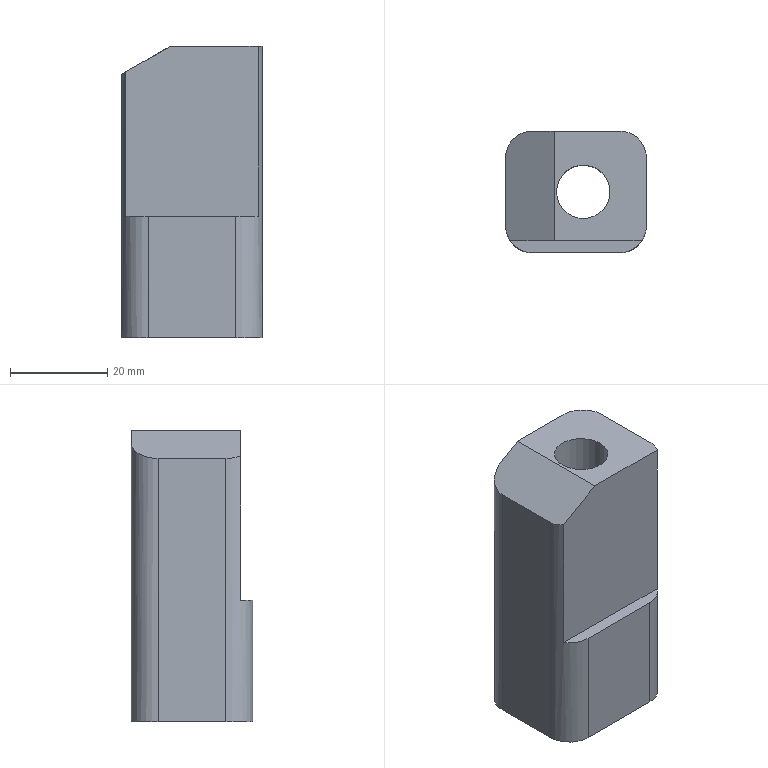Part | NX | features 1605338300 2 | 1 solid | 16 faces | box 29 x 25 x 60 mm | volume 29922 mm3 | plane 10 | cylinder 6 | commonest cylinder face diameters 11 x5 17 x1
STEP:
#1=CARTESIAN_POINT('',(321.5,0.000000002,-34.5));
#2=VERTEX_POINT('',#1);
#3=CARTESIAN_POINT('',(330.,0.000000002,-34.5));
#4=DIRECTION('',(0.,0.,-1.));
#5=DIRECTION('',(-1.,0.,0.));
#6=AXIS2_PLACEMENT_3D('',#3,#4,#5);
#7=CIRCLE('',#6,8.5);
#8=EDGE_CURVE('',#2,#2,#7,.T.);
#9=ORIENTED_EDGE('',*,*,#8,.F.);
#10=EDGE_LOOP('',(#9));
#11=FACE_BOUND('',#10,.T.);
#12=CARTESIAN_POINT('',(321.5,0.000000002,-61.5));
#13=VERTEX_POINT('',#12);
#14=CARTESIAN_POINT('',(330.,0.000000002,-61.5));
#15=DIRECTION('',(0.,0.,-1.));
#16=DIRECTION('',(-1.,0.,0.));
#17=AXIS2_PLACEMENT_3D('',#14,#15,#16);
#18=CIRCLE('',#17,8.5);
#19=EDGE_CURVE('',#13,#13,#18,.F.);
#20=ORIENTED_EDGE('',*,*,#19,.F.);
#21=EDGE_LOOP('',(#20));
#22=FACE_BOUND('',#21,.T.);
#23=CARTESIAN_POINT('',(330.,0.000000002,-34.5));
#24=DIRECTION('',(0.,0.,-1.));
#25=DIRECTION('',(-1.,0.,0.));
#26=AXIS2_PLACEMENT_3D('',#23,#24,#25);
#27=CYLINDRICAL_SURFACE('',#26,8.5);
#28=ADVANCED_FACE('',(#11,#22),#27,.F.);
#29=CARTESIAN_POINT('',(324.5,0.,-34.5));
#30=VERTEX_POINT('',#29);
#31=CARTESIAN_POINT('',(330.,0.,-34.5));
#32=DIRECTION('',(0.,0.,-1.));
#33=DIRECTION('',(-1.,0.,0.));
#34=AXIS2_PLACEMENT_3D('',#31,#32,#33);
#35=CIRCLE('',#34,5.5);
#36=EDGE_CURVE('',#30,#30,#35,.T.);
#37=ORIENTED_EDGE('',*,*,#36,.T.);
#38=EDGE_LOOP('',(#37));
#39=FACE_BOUND('',#38,.T.);
#40=CARTESIAN_POINT('',(335.5,0.,-1.5));
#41=VERTEX_POINT('',#40);
#42=CARTESIAN_POINT('',(330.,0.,-1.5));
#43=DIRECTION('',(0.,0.,1.));
#44=DIRECTION('',(1.,0.,0.));
#45=AXIS2_PLACEMENT_3D('',#42,#43,#44);
#46=CIRCLE('',#45,5.5);
#47=EDGE_CURVE('',#41,#41,#46,.F.);
#48=ORIENTED_EDGE('',*,*,#47,.F.);
#49=EDGE_LOOP('',(#48));
#50=FACE_BOUND('',#49,.T.);
#51=CARTESIAN_POINT('',(330.,0.,20.5));
#52=DIRECTION('',(0.,0.,-1.));
#53=DIRECTION('',(-1.,0.,0.));
#54=AXIS2_PLACEMENT_3D('',#51,#52,#53);
#55=CYLINDRICAL_SURFACE('',#54,5.5);
#56=ADVANCED_FACE('',(#39,#50),#55,.F.);
#57=CARTESIAN_POINT('',(324.,-10.,-1.5));
#58=VERTEX_POINT('',#57);
#59=CARTESIAN_POINT('',(324.,12.5,-1.5));
#60=VERTEX_POINT('',#59);
#61=CARTESIAN_POINT('',(324.,-5.,-1.5));
#62=DIRECTION('',(0.,1.,0.));
#63=VECTOR('',#62,1000.);
#64=LINE('',#61,#63);
#65=EDGE_CURVE('',#58,#60,#64,.T.);
#66=ORIENTED_EDGE('',*,*,#65,.F.);
#67=CARTESIAN_POINT('',(342.11,-10.,-1.5));
#68=VERTEX_POINT('',#67);
#69=CARTESIAN_POINT('',(326.,-10.,-1.5));
#70=DIRECTION('',(1.,0.,0.));
#71=VECTOR('',#70,1000.);
#72=LINE('',#69,#71);
#73=EDGE_CURVE('',#58,#68,#72,.T.);
#74=ORIENTED_EDGE('',*,*,#73,.T.);
#75=CARTESIAN_POINT('',(343.,-7.,-1.5));
#76=VERTEX_POINT('',#75);
#77=CARTESIAN_POINT('',(337.5,-7.,-1.5));
#78=DIRECTION('',(0.,0.,1.));
#79=DIRECTION('',(1.,0.,0.));
#80=AXIS2_PLACEMENT_3D('',#77,#78,#79);
#81=CIRCLE('',#80,5.5);
#82=EDGE_CURVE('',#76,#68,#81,.F.);
#83=ORIENTED_EDGE('',*,*,#82,.F.);
#84=CARTESIAN_POINT('',(343.,7.,-1.5));
#85=VERTEX_POINT('',#84);
#86=CARTESIAN_POINT('',(343.,-5.,-1.5));
#87=DIRECTION('',(0.,1.,0.));
#88=VECTOR('',#87,1000.);
#89=LINE('',#86,#88);
#90=EDGE_CURVE('',#76,#85,#89,.T.);
#91=ORIENTED_EDGE('',*,*,#90,.T.);
#92=CARTESIAN_POINT('',(337.5,12.5,-1.5));
#93=VERTEX_POINT('',#92);
#94=CARTESIAN_POINT('',(337.5,7.,-1.5));
#95=DIRECTION('',(0.,0.,1.));
#96=DIRECTION('',(1.,0.,0.));
#97=AXIS2_PLACEMENT_3D('',#94,#95,#96);
#98=CIRCLE('',#97,5.5);
#99=EDGE_CURVE('',#93,#85,#98,.F.);
#100=ORIENTED_EDGE('',*,*,#99,.F.);
#101=CARTESIAN_POINT('',(299.,12.5,-1.5));
#102=DIRECTION('',(-1.,0.,0.));
#103=VECTOR('',#102,1000.);
#104=LINE('',#101,#103);
#105=EDGE_CURVE('',#93,#60,#104,.T.);
#106=ORIENTED_EDGE('',*,*,#105,.T.);
#107=EDGE_LOOP('',(#66,#74,#83,#91,#100,#106));
#108=FACE_BOUND('',#107,.T.);
#109=ORIENTED_EDGE('',*,*,#47,.T.);
#110=EDGE_LOOP('',(#109));
#111=FACE_BOUND('',#110,.T.);
#112=CARTESIAN_POINT('',(299.,-5.,-1.5));
#113=DIRECTION('',(0.,0.,1.));
#114=DIRECTION('',(1.,0.,0.));
#115=AXIS2_PLACEMENT_3D('',#112,#113,#114);
#116=PLANE('',#115);
#117=ADVANCED_FACE('',(#108,#111),#116,.T.);
#118=CARTESIAN_POINT('',(337.5,-12.5,-36.5));
#119=VERTEX_POINT('',#118);
#120=CARTESIAN_POINT('',(319.5,-12.5,-36.5));
#121=VERTEX_POINT('',#120);
#122=CARTESIAN_POINT('',(326.,-12.5,-36.5));
#123=DIRECTION('',(1.,0.,0.));
#124=VECTOR('',#123,1000.);
#125=LINE('',#122,#124);
#126=EDGE_CURVE('',#119,#121,#125,.F.);
#127=ORIENTED_EDGE('',*,*,#126,.T.);
#128=CARTESIAN_POINT('',(319.5,-12.5,-61.5));
#129=VERTEX_POINT('',#128);
#130=CARTESIAN_POINT('',(319.5,-12.5,-1.5));
#131=DIRECTION('',(0.,0.,-1.));
#132=VECTOR('',#131,1000.);
#133=LINE('',#130,#132);
#134=EDGE_CURVE('',#129,#121,#133,.F.);
#135=ORIENTED_EDGE('',*,*,#134,.F.);
#136=CARTESIAN_POINT('',(337.5,-12.5,-61.5));
#137=VERTEX_POINT('',#136);
#138=CARTESIAN_POINT('',(299.,-12.5,-61.5));
#139=DIRECTION('',(-1.,0.,0.));
#140=VECTOR('',#139,1000.);
#141=LINE('',#138,#140);
#142=EDGE_CURVE('',#137,#129,#141,.T.);
#143=ORIENTED_EDGE('',*,*,#142,.F.);
#144=CARTESIAN_POINT('',(337.5,-12.5,-1.5));
#145=DIRECTION('',(0.,0.,-1.));
#146=VECTOR('',#145,1000.);
#147=LINE('',#144,#146);
#148=EDGE_CURVE('',#119,#137,#147,.T.);
#149=ORIENTED_EDGE('',*,*,#148,.F.);
#150=EDGE_LOOP('',(#127,#135,#143,#149));
#151=FACE_BOUND('',#150,.T.);
#152=CARTESIAN_POINT('',(299.,-12.5,-1.5));
#153=DIRECTION('',(0.,-1.,0.));
#154=DIRECTION('',(0.,0.,1.));
#155=AXIS2_PLACEMENT_3D('',#152,#153,#154);
#156=PLANE('',#155);
#157=ADVANCED_FACE('',(#151),#156,.T.);
#158=CARTESIAN_POINT('',(314.,7.,-7.274));
#159=VERTEX_POINT('',#158);
#160=CARTESIAN_POINT('',(314.,-7.,-7.274));
#161=VERTEX_POINT('',#160);
#162=CARTESIAN_POINT('',(314.,-5.,-7.274));
#163=DIRECTION('',(0.,1.,0.));
#164=VECTOR('',#163,1000.);
#165=LINE('',#162,#164);
#166=EDGE_CURVE('',#159,#161,#165,.F.);
#167=ORIENTED_EDGE('',*,*,#166,.F.);
#168=CARTESIAN_POINT('',(314.,7.,-61.5));
#169=VERTEX_POINT('',#168);
#170=CARTESIAN_POINT('',(314.,7.,-1.5));
#171=DIRECTION('',(0.,0.,-1.));
#172=VECTOR('',#171,1000.);
#173=LINE('',#170,#172);
#174=EDGE_CURVE('',#169,#159,#173,.F.);
#175=ORIENTED_EDGE('',*,*,#174,.F.);
#176=CARTESIAN_POINT('',(314.,-7.,-61.5));
#177=VERTEX_POINT('',#176);
#178=CARTESIAN_POINT('',(314.,-5.,-61.5));
#179=DIRECTION('',(0.,1.,0.));
#180=VECTOR('',#179,1000.);
#181=LINE('',#178,#180);
#182=EDGE_CURVE('',#177,#169,#181,.T.);
#183=ORIENTED_EDGE('',*,*,#182,.F.);
#184=CARTESIAN_POINT('',(314.,-7.,-1.5));
#185=DIRECTION('',(0.,0.,-1.));
#186=VECTOR('',#185,1000.);
#187=LINE('',#184,#186);
#188=EDGE_CURVE('',#161,#177,#187,.T.);
#189=ORIENTED_EDGE('',*,*,#188,.F.);
#190=EDGE_LOOP('',(#167,#175,#183,#189));
#191=FACE_BOUND('',#190,.T.);
#192=CARTESIAN_POINT('',(314.,-5.,-1.5));
#193=DIRECTION('',(-1.,0.,0.));
#194=DIRECTION('',(0.,0.,1.));
#195=AXIS2_PLACEMENT_3D('',#192,#193,#194);
#196=PLANE('',#195);
#197=ADVANCED_FACE('',(#191),#196,.T.);
#198=CARTESIAN_POINT('',(319.5,12.5,-4.098));
#199=VERTEX_POINT('',#198);
#200=CARTESIAN_POINT('',(301.5,12.5,-14.49));
#201=DIRECTION('',(-0.866,0.,-0.5));
#202=VECTOR('',#201,1000.);
#203=LINE('',#200,#202);
#204=EDGE_CURVE('',#60,#199,#203,.T.);
#205=ORIENTED_EDGE('',*,*,#204,.F.);
#206=ORIENTED_EDGE('',*,*,#105,.F.);
#207=CARTESIAN_POINT('',(337.5,12.5,-61.5));
#208=VERTEX_POINT('',#207);
#209=CARTESIAN_POINT('',(337.5,12.5,-1.5));
#210=DIRECTION('',(0.,0.,-1.));
#211=VECTOR('',#210,1000.);
#212=LINE('',#209,#211);
#213=EDGE_CURVE('',#208,#93,#212,.F.);
#214=ORIENTED_EDGE('',*,*,#213,.F.);
#215=CARTESIAN_POINT('',(319.5,12.5,-61.5));
#216=VERTEX_POINT('',#215);
#217=CARTESIAN_POINT('',(299.,12.5,-61.5));
#218=DIRECTION('',(1.,0.,0.));
#219=VECTOR('',#218,1000.);
#220=LINE('',#217,#219);
#221=EDGE_CURVE('',#216,#208,#220,.T.);
#222=ORIENTED_EDGE('',*,*,#221,.F.);
#223=CARTESIAN_POINT('',(319.5,12.5,-1.5));
#224=DIRECTION('',(0.,0.,-1.));
#225=VECTOR('',#224,1000.);
#226=LINE('',#223,#225);
#227=EDGE_CURVE('',#199,#216,#226,.T.);
#228=ORIENTED_EDGE('',*,*,#227,.F.);
#229=EDGE_LOOP('',(#205,#206,#214,#222,#228));
#230=FACE_BOUND('',#229,.T.);
#231=CARTESIAN_POINT('',(299.,12.5,-1.5));
#232=DIRECTION('',(0.,1.,0.));
#233=DIRECTION('',(0.,0.,-1.));
#234=AXIS2_PLACEMENT_3D('',#231,#232,#233);
#235=PLANE('',#234);
#236=ADVANCED_FACE('',(#230),#235,.T.);
#237=CARTESIAN_POINT('',(343.,7.,-61.5));
#238=VERTEX_POINT('',#237);
#239=CARTESIAN_POINT('',(343.,-7.,-61.5));
#240=VERTEX_POINT('',#239);
#241=CARTESIAN_POINT('',(343.,-5.,-61.5));
#242=DIRECTION('',(0.,-1.,0.));
#243=VECTOR('',#242,1000.);
#244=LINE('',#241,#243);
#245=EDGE_CURVE('',#238,#240,#244,.T.);
#246=ORIENTED_EDGE('',*,*,#245,.F.);
#247=CARTESIAN_POINT('',(343.,7.,-1.5));
#248=DIRECTION('',(0.,0.,-1.));
#249=VECTOR('',#248,1000.);
#250=LINE('',#247,#249);
#251=EDGE_CURVE('',#85,#238,#250,.T.);
#252=ORIENTED_EDGE('',*,*,#251,.F.);
#253=ORIENTED_EDGE('',*,*,#90,.F.);
#254=CARTESIAN_POINT('',(343.,-7.,-1.5));
#255=DIRECTION('',(0.,0.,-1.));
#256=VECTOR('',#255,1000.);
#257=LINE('',#254,#256);
#258=EDGE_CURVE('',#240,#76,#257,.F.);
#259=ORIENTED_EDGE('',*,*,#258,.F.);
#260=EDGE_LOOP('',(#246,#252,#253,#259));
#261=FACE_BOUND('',#260,.T.);
#262=CARTESIAN_POINT('',(343.,-5.,-1.5));
#263=DIRECTION('',(1.,0.,0.));
#264=DIRECTION('',(0.,0.,-1.));
#265=AXIS2_PLACEMENT_3D('',#262,#263,#264);
#266=PLANE('',#265);
#267=ADVANCED_FACE('',(#261),#266,.T.);
#268=CARTESIAN_POINT('',(314.89,-10.,-6.76));
#269=VERTEX_POINT('',#268);
#270=CARTESIAN_POINT('',(314.,-10.,-7.274));
#271=DIRECTION('',(0.866,0.,0.5));
#272=VECTOR('',#271,1000.);
#273=LINE('',#270,#272);
#274=EDGE_CURVE('',#58,#269,#273,.F.);
#275=ORIENTED_EDGE('',*,*,#274,.F.);
#276=ORIENTED_EDGE('',*,*,#65,.T.);
#277=ORIENTED_EDGE('',*,*,#204,.T.);
#278=CARTESIAN_POINT('',(319.5,7.,-4.098));
#279=DIRECTION('',(0.5,0.,-0.866));
#280=DIRECTION('',(0.866,0.,0.5));
#281=AXIS2_PLACEMENT_3D('',#278,#279,#280);
#282=ELLIPSE('',#281,6.351,5.5);
#283=EDGE_CURVE('',#159,#199,#282,.T.);
#284=ORIENTED_EDGE('',*,*,#283,.F.);
#285=ORIENTED_EDGE('',*,*,#166,.T.);
#286=CARTESIAN_POINT('',(319.5,-7.,-4.098));
#287=DIRECTION('',(0.5,0.,-0.866));
#288=DIRECTION('',(0.866,0.,0.5));
#289=AXIS2_PLACEMENT_3D('',#286,#287,#288);
#290=ELLIPSE('',#289,6.351,5.5);
#291=EDGE_CURVE('',#269,#161,#290,.T.);
#292=ORIENTED_EDGE('',*,*,#291,.F.);
#293=EDGE_LOOP('',(#275,#276,#277,#284,#285,#292));
#294=FACE_BOUND('',#293,.T.);
#295=CARTESIAN_POINT('',(314.,-5.,-7.274));
#296=DIRECTION('',(0.5,0.,-0.866));
#297=DIRECTION('',(-0.866,0.,-0.5));
#298=AXIS2_PLACEMENT_3D('',#295,#296,#297);
#299=PLANE('',#298);
#300=ADVANCED_FACE('',(#294),#299,.F.);
#301=ORIENTED_EDGE('',*,*,#99,.T.);
#302=ORIENTED_EDGE('',*,*,#251,.T.);
#303=CARTESIAN_POINT('',(337.5,7.,-61.5));
#304=DIRECTION('',(0.,0.,-1.));
#305=DIRECTION('',(-1.,0.,0.));
#306=AXIS2_PLACEMENT_3D('',#303,#304,#305);
#307=CIRCLE('',#306,5.5);
#308=EDGE_CURVE('',#238,#208,#307,.F.);
#309=ORIENTED_EDGE('',*,*,#308,.T.);
#310=ORIENTED_EDGE('',*,*,#213,.T.);
#311=EDGE_LOOP('',(#301,#302,#309,#310));
#312=FACE_BOUND('',#311,.T.);
#313=CARTESIAN_POINT('',(337.5,7.,-1.5));
#314=DIRECTION('',(0.,0.,1.));
#315=DIRECTION('',(1.,0.,0.));
#316=AXIS2_PLACEMENT_3D('',#313,#314,#315);
#317=CYLINDRICAL_SURFACE('',#316,5.5);
#318=ADVANCED_FACE('',(#312),#317,.T.);
#319=CARTESIAN_POINT('',(342.11,-10.,-36.5));
#320=VERTEX_POINT('',#319);
#321=CARTESIAN_POINT('',(337.5,-7.,-36.5));
#322=DIRECTION('',(0.,0.,1.));
#323=DIRECTION('',(1.,0.,0.));
#324=AXIS2_PLACEMENT_3D('',#321,#322,#323);
#325=CIRCLE('',#324,5.5);
#326=EDGE_CURVE('',#320,#119,#325,.F.);
#327=ORIENTED_EDGE('',*,*,#326,.T.);
#328=ORIENTED_EDGE('',*,*,#148,.T.);
#329=CARTESIAN_POINT('',(337.5,-7.,-61.5));
#330=DIRECTION('',(0.,0.,-1.));
#331=DIRECTION('',(-1.,0.,0.));
#332=AXIS2_PLACEMENT_3D('',#329,#330,#331);
#333=CIRCLE('',#332,5.5);
#334=EDGE_CURVE('',#137,#240,#333,.F.);
#335=ORIENTED_EDGE('',*,*,#334,.T.);
#336=ORIENTED_EDGE('',*,*,#258,.T.);
#337=ORIENTED_EDGE('',*,*,#82,.T.);
#338=CARTESIAN_POINT('',(342.11,-10.,-1.5));
#339=DIRECTION('',(0.,0.,1.));
#340=VECTOR('',#339,1000.);
#341=LINE('',#338,#340);
#342=EDGE_CURVE('',#68,#320,#341,.F.);
#343=ORIENTED_EDGE('',*,*,#342,.T.);
#344=EDGE_LOOP('',(#327,#328,#335,#336,#337,#343));
#345=FACE_BOUND('',#344,.T.);
#346=CARTESIAN_POINT('',(337.5,-7.,-1.5));
#347=DIRECTION('',(0.,0.,1.));
#348=DIRECTION('',(1.,0.,0.));
#349=AXIS2_PLACEMENT_3D('',#346,#347,#348);
#350=CYLINDRICAL_SURFACE('',#349,5.5);
#351=ADVANCED_FACE('',(#345),#350,.T.);
#352=ORIENTED_EDGE('',*,*,#283,.T.);
#353=ORIENTED_EDGE('',*,*,#227,.T.);
#354=CARTESIAN_POINT('',(319.5,7.,-61.5));
#355=DIRECTION('',(0.,0.,-1.));
#356=DIRECTION('',(-1.,0.,0.));
#357=AXIS2_PLACEMENT_3D('',#354,#355,#356);
#358=CIRCLE('',#357,5.5);
#359=EDGE_CURVE('',#216,#169,#358,.F.);
#360=ORIENTED_EDGE('',*,*,#359,.T.);
#361=ORIENTED_EDGE('',*,*,#174,.T.);
#362=EDGE_LOOP('',(#352,#353,#360,#361));
#363=FACE_BOUND('',#362,.T.);
#364=CARTESIAN_POINT('',(319.5,7.,-1.5));
#365=DIRECTION('',(0.,0.,1.));
#366=DIRECTION('',(1.,0.,0.));
#367=AXIS2_PLACEMENT_3D('',#364,#365,#366);
#368=CYLINDRICAL_SURFACE('',#367,5.5);
#369=ADVANCED_FACE('',(#363),#368,.T.);
#370=CARTESIAN_POINT('',(314.89,-10.,-36.5));
#371=VERTEX_POINT('',#370);
#372=CARTESIAN_POINT('',(319.5,-7.,-36.5));
#373=DIRECTION('',(0.,0.,1.));
#374=DIRECTION('',(1.,0.,0.));
#375=AXIS2_PLACEMENT_3D('',#372,#373,#374);
#376=CIRCLE('',#375,5.5);
#377=EDGE_CURVE('',#121,#371,#376,.F.);
#378=ORIENTED_EDGE('',*,*,#377,.T.);
#379=CARTESIAN_POINT('',(314.89,-10.,-6.76));
#380=DIRECTION('',(0.,0.,1.));
#381=VECTOR('',#380,1000.);
#382=LINE('',#379,#381);
#383=EDGE_CURVE('',#269,#371,#382,.F.);
#384=ORIENTED_EDGE('',*,*,#383,.F.);
#385=ORIENTED_EDGE('',*,*,#291,.T.);
#386=ORIENTED_EDGE('',*,*,#188,.T.);
#387=CARTESIAN_POINT('',(319.5,-7.,-61.5));
#388=DIRECTION('',(0.,0.,-1.));
#389=DIRECTION('',(-1.,0.,0.));
#390=AXIS2_PLACEMENT_3D('',#387,#388,#389);
#391=CIRCLE('',#390,5.5);
#392=EDGE_CURVE('',#177,#129,#391,.F.);
#393=ORIENTED_EDGE('',*,*,#392,.T.);
#394=ORIENTED_EDGE('',*,*,#134,.T.);
#395=EDGE_LOOP('',(#378,#384,#385,#386,#393,#394));
#396=FACE_BOUND('',#395,.T.);
#397=CARTESIAN_POINT('',(319.5,-7.,-1.5));
#398=DIRECTION('',(0.,0.,1.));
#399=DIRECTION('',(1.,0.,0.));
#400=AXIS2_PLACEMENT_3D('',#397,#398,#399);
#401=CYLINDRICAL_SURFACE('',#400,5.5);
#402=ADVANCED_FACE('',(#396),#401,.T.);
#403=ORIENTED_EDGE('',*,*,#8,.T.);
#404=EDGE_LOOP('',(#403));
#405=FACE_BOUND('',#404,.T.);
#406=ORIENTED_EDGE('',*,*,#36,.F.);
#407=EDGE_LOOP('',(#406));
#408=FACE_BOUND('',#407,.T.);
#409=CARTESIAN_POINT('',(280.,-64.5,-34.5));
#410=DIRECTION('',(0.,0.,-1.));
#411=DIRECTION('',(-1.,0.,0.));
#412=AXIS2_PLACEMENT_3D('',#409,#410,#411);
#413=PLANE('',#412);
#414=ADVANCED_FACE('',(#405,#408),#413,.T.);
#415=ORIENTED_EDGE('',*,*,#182,.T.);
#416=ORIENTED_EDGE('',*,*,#359,.F.);
#417=ORIENTED_EDGE('',*,*,#221,.T.);
#418=ORIENTED_EDGE('',*,*,#308,.F.);
#419=ORIENTED_EDGE('',*,*,#245,.T.);
#420=ORIENTED_EDGE('',*,*,#334,.F.);
#421=ORIENTED_EDGE('',*,*,#142,.T.);
#422=ORIENTED_EDGE('',*,*,#392,.F.);
#423=EDGE_LOOP('',(#415,#416,#417,#418,#419,#420,#421,#422));
#424=FACE_BOUND('',#423,.T.);
#425=ORIENTED_EDGE('',*,*,#19,.T.);
#426=EDGE_LOOP('',(#425));
#427=FACE_BOUND('',#426,.T.);
#428=CARTESIAN_POINT('',(299.,-5.,-61.5));
#429=DIRECTION('',(0.,0.,-1.));
#430=DIRECTION('',(-1.,0.,0.));
#431=AXIS2_PLACEMENT_3D('',#428,#429,#430);
#432=PLANE('',#431);
#433=ADVANCED_FACE('',(#424,#427),#432,.T.);
#434=ORIENTED_EDGE('',*,*,#73,.F.);
#435=ORIENTED_EDGE('',*,*,#274,.T.);
#436=ORIENTED_EDGE('',*,*,#383,.T.);
#437=CARTESIAN_POINT('',(326.,-10.,-36.5));
#438=DIRECTION('',(1.,0.,0.));
#439=VECTOR('',#438,1000.);
#440=LINE('',#437,#439);
#441=EDGE_CURVE('',#371,#320,#440,.T.);
#442=ORIENTED_EDGE('',*,*,#441,.T.);
#443=ORIENTED_EDGE('',*,*,#342,.F.);
#444=EDGE_LOOP('',(#434,#435,#436,#442,#443));
#445=FACE_BOUND('',#444,.T.);
#446=CARTESIAN_POINT('',(326.,-10.,-36.5));
#447=DIRECTION('',(0.,1.,0.));
#448=DIRECTION('',(0.,0.,1.));
#449=AXIS2_PLACEMENT_3D('',#446,#447,#448);
#450=PLANE('',#449);
#451=ADVANCED_FACE('',(#445),#450,.F.);
#452=ORIENTED_EDGE('',*,*,#126,.F.);
#453=ORIENTED_EDGE('',*,*,#326,.F.);
#454=ORIENTED_EDGE('',*,*,#441,.F.);
#455=ORIENTED_EDGE('',*,*,#377,.F.);
#456=EDGE_LOOP('',(#452,#453,#454,#455));
#457=FACE_BOUND('',#456,.T.);
#458=CARTESIAN_POINT('',(322.,-12.5,-36.5));
#459=DIRECTION('',(0.,0.,1.));
#460=DIRECTION('',(1.,0.,0.));
#461=AXIS2_PLACEMENT_3D('',#458,#459,#460);
#462=PLANE('',#461);
#463=ADVANCED_FACE('',(#457),#462,.T.);
#464=CLOSED_SHELL('',(#28,#56,#117,#157,#197,#236,#267,#300,#318,#351,#369,#402,#414,#433,#451,#463));
#465=MANIFOLD_SOLID_BREP('',#464);
#466=(LENGTH_UNIT()NAMED_UNIT(*)SI_UNIT(.MILLI.,.METRE.));
#467=UNCERTAINTY_MEASURE_WITH_UNIT(LENGTH_MEASURE(0.00001),#466,'','');
#468=(NAMED_UNIT(*)PLANE_ANGLE_UNIT()SI_UNIT($,.RADIAN.));
#469=(NAMED_UNIT(*)SI_UNIT($,.STERADIAN.)SOLID_ANGLE_UNIT());
#470=(GEOMETRIC_REPRESENTATION_CONTEXT(3)GLOBAL_UNCERTAINTY_ASSIGNED_CONTEXT((#467))GLOBAL_UNIT_ASSIGNED_CONTEXT((#466,#468,#469))REPRESENTATION_CONTEXT('',''));
#471=ADVANCED_BREP_SHAPE_REPRESENTATION('',(#465),#470);